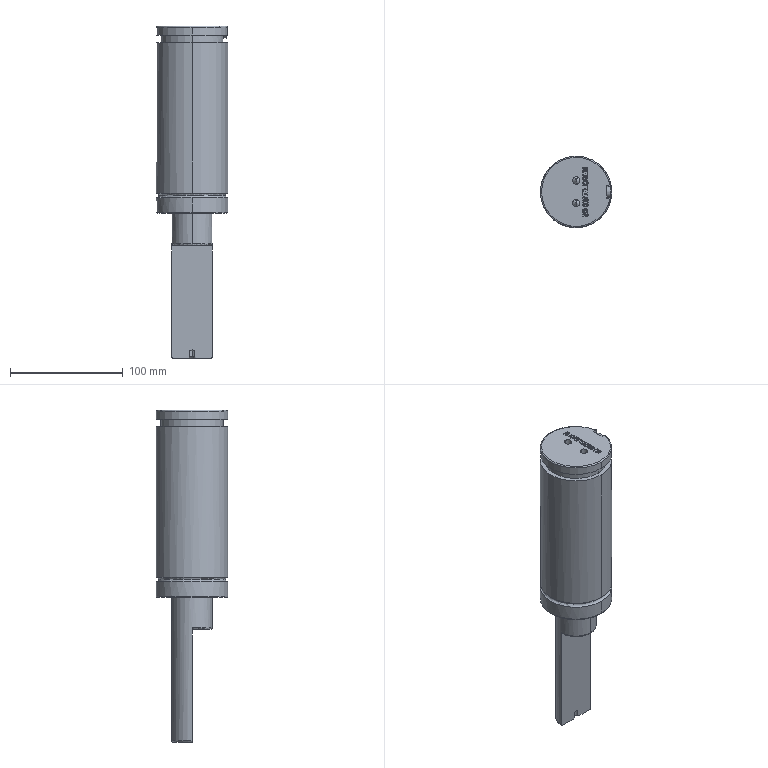Part | STEP file | 1_id2310_x_t | 1 solid | 220 faces | box 63.2 x 63.2 x 294 mm | volume 592651 mm3 | plane 143 | other 37 | cylinder 22 | cone 12 | torus 6 | commonest cylinder face diameters 63.2 x7 4.9 x4 6.6 x4 9.5 x2 36 x2 55.6 x2